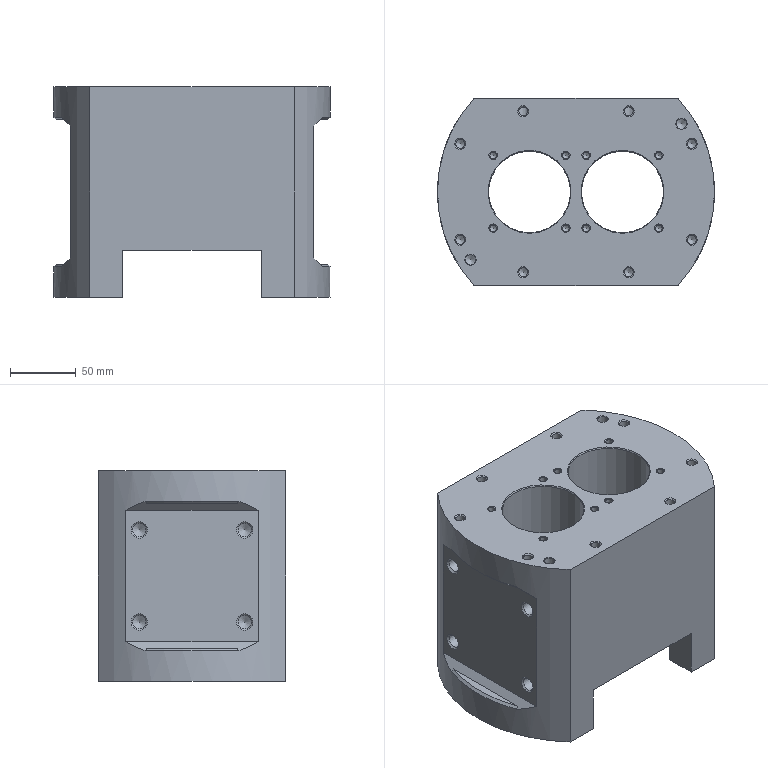NC program | NX | posted with a generic post | part box 210 x 142 x 160 mm
Whole program:
N10 G17 G21 G94 G90
(FLOOR_WALL , TOOL : D50)
N12 T02 M6
N14 G54
N16 G17 G0 G90 X-46.563 Y89.997 B0. C0. S1200 M3
N18 G43 Z30. H2
N20 Z2.65
N22 G94 G1 Z-0.35 F1000.
N24 X-43.563
N26 X43.563 F2000.
N28 Y49.998
N30 X-43.563
N32 Y9.999
N34 X43.563
N36 Y-30.001
N38 X-43.563
N40 Y-70.
N42 X43.563
N44 X46.563
N46 Z2.65
N48 G0 Z30.
N50 X-50.098 Y89.997
N52 Z2.301
N54 G1 Z-0.699 F1000.
N56 X-47.098
N58 X47.098 F2000.
N60 Y49.998
N62 X-47.098
N64 Y9.999
N66 X47.098
N68 Y-30.001
N70 X-47.098
N72 Y-70.
N74 X47.098
N76 X50.098
N78 Z2.301
N80 G0 Z30.
N82 X-52.803 Y89.997
N84 Z1.951
N86 G1 Z-1.049 F1000.
N88 X-49.803
N90 X49.803 F2000.
N92 Y49.998
N94 X-49.803
N96 Y9.999
N98 X49.803
N100 Y-30.001
N102 X-49.803
N104 Y-70.
N106 X49.803
N108 X52.803
N110 Z1.951
N112 G0 Z30.
N114 X-55.078 Y89.997
N116 Z1.602
N118 G1 Z-1.398 F1000.
N120 X-52.078
N122 X52.078 F2000.
N124 Y49.998
N126 X-52.078
N128 Y9.999
N130 X52.078
N132 Y-30.001
N134 X-52.078
N136 Y-70.
N138 X52.078
N140 X55.078
N142 Z1.602
N144 G0 Z30.
N146 X-57.078 Y89.997
N148 Z1.252
N150 G1 Z-1.748 F1000.
N152 X-54.078
N154 X54.078 F2000.
N156 Y49.998
N158 X-54.078
N160 Y9.999
N162 X54.078
N164 Y-30.001
N166 X-54.078
N168 Y-70.
N170 X54.078
N172 X57.078
N174 Z1.252
N176 G0 Z30.
N178 X-58.881 Y89.997
N180 Z0.903
N182 G1 Z-2.097 F1000.
N184 X-55.881
N186 X55.881 F2000.
N188 Y49.998
N190 X-55.881
N192 Y9.999
N194 X55.881
N196 Y-30.001
N198 X-55.881
N200 Y-70.
N202 X55.881
N204 X58.881
N206 Z0.903
N208 G0 Z30.
N210 X-60.535 Y89.997
N212 Z0.553
N214 G1 Z-2.447 F1000.
N216 X-57.535
N218 X57.535 F2000.
N220 Y49.998
N222 X-57.535
N224 Y9.999
N226 X57.535
N228 Y-30.001
N230 X-57.535
N232 Y-70.
N234 X57.535
N236 X60.535
N238 Z0.553
N240 G0 Z30.
N242 X-62.07 Y89.997
N244 Z0.204
N246 G1 Z-2.796 F1000.
N248 X-59.07
N250 X59.07 F2000.
N252 Y49.998
N254 X-59.07
N256 Y9.999
N258 X59.07
N260 Y-30.001
N262 X-59.07
N264 Y-70.
N266 X59.07
N268 X62.07
N270 Z0.204
N272 G0 Z30.
N274 X-63.509 Y89.997
N276 Z-0.146
N278 G1 Z-3.146 F1000.
N280 X-60.509
N282 X60.509 F2000.
N284 Y49.998
N286 X-60.509
N288 Y9.999
N290 X60.509
N292 Y-30.001
N294 X-60.509
N296 Y-70.
N298 X60.509
N300 X63.509
N302 Z-0.146
N304 G0 Z30.
N306 X-64.866 Y89.997
N308 Z-0.495
N310 G1 Z-3.495 F1000.
N312 X-61.866
N314 X61.866 F2000.
N316 Y49.998
N318 X-61.866
N320 Y9.999
N322 X61.866
N324 Y-30.001
N326 X-61.866
N328 Y-70.
N330 X61.866
N332 X64.866
N334 Z-0.495
N336 G0 Z30.
N338 X-66.153 Y89.997
N340 Z-0.845
N342 G1 Z-3.845 F1000.
N344 X-63.153
N346 X63.153 F2000.
N348 Y49.998
N350 X-63.153
N352 Y9.999
N354 X63.153
N356 Y-30.001
N358 X-63.153
N360 Y-70.
N362 X63.153
N364 X66.153
N366 Z-0.845
N368 G0 Z30.
N370 X-67.38 Y89.997
N372 Z-1.194
N374 G1 Z-4.194 F1000.
N376 X-64.38
N378 X64.38 F2000.
N380 Y49.998
N382 X-64.38
N384 Y9.999
N386 X64.38
N388 Y-30.001
N390 X-64.38
N392 Y-70.
N394 X64.38
N396 X67.38
N398 Z-1.194
N400 G0 Z30.
N402 X-68.553 Y89.997
N404 Z-1.544
N406 G1 Z-4.544 F1000.
N408 X-65.553
N410 X65.553 F2000.
N412 Y49.998
N414 X-65.553
N416 Y9.999
N418 X65.553
N420 Y-30.001
N422 X-65.553
N424 Y-70.
N426 X65.553
N428 X68.553
N430 Z-1.544
N432 G0 Z30.
N434 X-69.68 Y89.997
N436 Z-1.893
N438 G1 Z-4.893 F1000.
N440 X-66.68
N442 X66.68 F2000.
N444 Y49.998
N446 X-66.68
N448 Y9.999
N450 X66.68
N452 Y-30.001
N454 X-66.68
N456 Y-70.
N458 X66.68
N460 X69.68
N462 Z-1.893
N464 G0 Z30.
N466 X-70.763 Y89.997
N468 Z-2.243
N470 G1 Z-5.243 F1000.
N472 X-67.763
N474 X67.763 F2000.
N476 Y49.998
N478 X-67.763
N480 Y9.999
N482 X67.763
N484 Y-30.001
N486 X-67.763
N488 Y-70.
N490 X67.763
N492 X70.763
N494 Z-2.243
N496 G0 Z30.
N498 X-71.809 Y89.997
N500 Z-2.592
N502 G1 Z-5.592 F1000.
N504 X-68.809
N506 X68.809 F2000.
N508 Y49.998
N510 X-68.809
N512 Y9.999
N514 X68.809
N516 Y-30.001
N518 X-68.809
N520 Y-70.
N522 X68.809
N524 X71.809
N526 Z-2.592
N528 G0 Z30.
N530 X-72.82 Y89.997
N532 Z-2.941
N534 G1 Z-5.941 F1000.
N536 X-69.82
N538 X69.82 F2000.
N540 Y49.998
N542 X-69.82
N544 Y9.999
N546 X69.82
N548 Y-30.001
N550 X-69.82
N552 Y-70.
N554 X69.82
N556 X72.82
N558 Z-2.941
N560 G0 Z30.
N562 X-73.798 Y89.997
N564 Z-3.291
N566 G1 Z-6.291 F1000.
N568 X-70.798
N570 X70.798 F2000.
N572 Y49.998
N574 X-70.798
N576 Y9.999
N578 X70.798
N580 Y-30.001
N582 X-70.798
N584 Y-70.
N586 X70.798
N588 X73.798
N590 Z-3.291
N592 G0 Z30.
N594 X-74.748 Y89.997
N596 Z-3.64
N598 G1 Z-6.64 F1000.
N600 X-71.748
N602 X71.748 F2000.
N604 Y49.998
N606 X-71.748
N608 Y9.999
N610 X71.748
N612 Y-30.001
N614 X-71.748
N616 Y-70.
N618 X71.748
N620 X74.748
N622 Z-3.64
N624 G0 Z30.
N626 X-75.67 Y89.997
N628 Z-3.99
N630 G1 Z-6.99 F1000.
N632 X-72.67
N634 X72.67 F2000.
N636 Y49.998
N638 X-72.67
N640 Y9.999
N642 X72.67
N644 Y-30.001
N646 X-72.67
N648 Y-70.
N650 X72.67
N652 X75.67
N654 Z-3.99
N656 G0 Z30.
N658 X-76.567 Y89.997
N660 Z-4.339
N662 G1 Z-7.339 F1000.
N664 X-73.567
N666 X73.567 F2000.
N668 Y49.998
N670 X-73.567
N672 Y9.999
N674 X73.567
N676 Y-30.001
N678 X-73.567
N680 Y-70.
N682 X73.567
N684 X76.567
N686 Z-4.339
N688 G0 Z30.
N690 X-77.44 Y89.997
N692 Z-4.689
N694 G1 Z-7.689 F1000.
N696 X-74.44
N698 X74.44 F2000.
N700 Y49.998
N702 X-74.44
N704 Y9.999
N706 X74.44
N708 Y-30.001
N710 X-74.44
N712 Y-70.
N714 X74.44
N716 X77.44
N718 Z-4.689
N720 G0 Z30.
N722 X-78.292 Y89.997
N724 Z-5.038
N726 G1 Z-8.038 F1000.
N728 X-75.292
N730 X75.292 F2000.
N732 Y49.998
N734 X-75.292
N736 Y9.999
N738 X75.292
N740 Y-30.001
N742 X-75.292
N744 Y-70.
N746 X75.292
N748 X78.292
N750 Z-5.038
N752 G0 Z30.
N754 X-79.123 Y89.997
N756 Z-5.388
N758 G1 Z-8.388 F1000.
N760 X-76.123
N762 X76.123 F2000.
N764 Y49.998
N766 X-76.123
N768 Y9.999
N770 X76.123
N772 Y-30.001
N774 X-76.123
N776 Y-70.
N778 X76.123
N780 X79.123
N782 Z-5.388
N784 G0 Z30.
N786 X-79.934 Y89.997
N788 Z-5.737
N790 G1 Z-8.737 F1000.
N792 X-76.934
N794 X76.934 F2000.
N796 Y49.998
N798 X-76.934
N800 Y9.999
N802 X76.934
N804 Y-30.001
N806 X-76.934
N808 Y-70.
N810 X76.934
N812 X79.934
N814 Z-5.737
N816 G0 Z30.
N818 X-80.728 Y89.997
N820 Z-6.087
N822 G1 Z-9.087 F1000.
N824 X-77.728
N826 X77.728 F2000.
N828 Y49.998
N830 X-77.728
N832 Y9.999
N834 X77.728
N836 Y-30.001
N838 X-77.728
N840 Y-70.
N842 X77.728
N844 X80.728
N846 Z-6.087
N848 G0 Z30.
N850 X-81.504 Y89.997
N852 Z-6.436
N854 G1 Z-9.436 F1000.
N856 X-78.504
N858 X78.504 F2000.
N860 Y49.998
N862 X-78.504
N864 Y9.999
N866 X78.504
N868 Y-30.001
N870 X-78.504
N872 Y-70.
N874 X78.504
N876 X81.504
N878 Z-6.436
N880 G0 Z30.
N882 X-82.263 Y89.997
N884 Z-6.786
N886 G1 Z-9.786 F1000.
N888 X-79.263
N890 X79.263 F2000.
N892 Y49.998
N894 X-79.263
N896 Y9.999
N898 X79.263
N900 Y-30.001
N902 X-79.263
N904 Y-70.
N906 X79.263
N908 X82.263
N910 Z-6.786
N912 G0 Z30.
N914 X-83.008 Y89.997
N916 Z-7.135
N918 G1 Z-10.135 F1000.
N920 X-80.008
N922 X80.008 F2000.
N924 Y49.998
N926 X-80.008
N928 Y9.999
N930 X80.008
N932 Y-30.001
N934 X-80.008
N936 Y-70.
N938 X80.008
N940 X83.008
N942 Z-7.135
N944 G0 Z30.
N946 X-83.737 Y89.997
N948 Z-7.485
N950 G1 Z-10.485 F1000.
N952 X-80.737
N954 X80.737 F2000.
N956 Y49.998
N958 X-80.737
N960 Y9.999
N962 X80.737
N964 Y-30.001
N966 X-80.737
N968 Y-70.
N970 X80.737
N972 X83.737
N974 Z-7.485
N976 G0 Z30.
N978 X-84.452 Y89.997
N980 Z-7.834
N982 G1 Z-10.834 F1000.
N984 X-81.452
N986 X81.452 F2000.
N988 Y49.998
N990 X-81.452
N992 Y9.999
N994 X81.452
N996 Y-30.001
N998 X-81.452
N1000 Y-70.
N1002 X81.452
N1004 X84.452
N1006 Z-7.834
N1008 G0 Z30.
N1010 X-85.154 Y89.997
N1012 Z-8.184
N1014 G1 Z-11.184 F1000.
N1016 X-82.154
N1018 X82.154 F2000.
N1020 Y49.998
N1022 X-82.154
N1024 Y9.999
N1026 X82.154
N1028 Y-30.001
N1030 X-82.154
N1032 Y-70.
N1034 X82.154
N1036 X85.154
N1038 Z-8.184
N1040 G0 Z30.
N1042 X-85.843 Y89.997
N1044 Z-8.533
N1046 G1 Z-11.533 F1000.
N1048 X-82.843
N1050 X82.843 F2000.
N1052 Y49.998
N1054 X-82.843
N1056 Y9.999
N1058 X82.843
N1060 Y-30.001
N1062 X-82.843
N1064 Y-70.
N1066 X82.843
N1068 X85.843
N1070 Z-8.533
N1072 G0 Z30.
N1074 X-86.52 Y89.997
N1076 Z-8.883
N1078 G1 Z-11.883 F1000.
N1080 X-83.52
N1082 X83.52 F2000.
N1084 Y49.998
N1086 X-83.52
N1088 Y9.999
N1090 X83.52
N1092 Y-30.001
N1094 X-83.52
N1096 Y-70.
N1098 X83.52
N1100 X86.52
N1102 Z-8.883
N1104 G0 Z30.
N1106 X-87.185 Y89.997
N1108 Z-9.232
N1110 G1 Z-12.232 F1000.
N1112 X-84.185
N1114 X84.185 F2000.
N1116 Y49.998
N1118 X-84.185
N1120 Y9.999
N1122 X84.185
N1124 Y-30.001
N1126 X-84.185
N1128 Y-70.
N1130 X84.185
N1132 X87.185
N1134 Z-9.232
N1136 G0 Z30.
N1138 X-87.838 Y89.997
N1140 Z-9.582
N1142 G1 Z-12.582 F1000.
N1144 X-84.838
N1146 X84.838 F2000.
N1148 Y49.998
N1150 X-84.838
N1152 Y9.999
N1154 X84.838
N1156 Y-30.001
N1158 X-84.838
N1160 Y-70.
N1162 X84.838
N1164 X87.838
N1166 Z-9.582
N1168 G0 Z30.
N1170 X-88.481 Y89.997
N1172 Z-9.931
N1174 G1 Z-12.931 F1000.
N1176 X-85.481
N1178 X85.481 F2000.
N1180 Y49.998
N1182 X-85.481
N1184 Y9.999
N1186 X85.481
N1188 Y-30.001
N1190 X-85.481
N1192 Y-70.
N1194 X85.481
N1196 X88.481
N1198 Z-9.931
N1200 G0 Z30.
N1202 X-89.113 Y89.997
N1204 Z-10.281
N1206 G1 Z-13.281 F1000.
N1208 X-86.113
N1210 X86.113 F2000.
N1212 Y49.998
N1214 X-86.113
N1216 Y9.999
N1218 X86.113
N1220 Y-30.001
N1222 X-86.113
N1224 Y-70.
N1226 X86.113
N1228 X89.113
N1230 Z-10.281
N1232 G0 Z30.
N1234 X-89.735 Y89.997
N1236 Z-10.63
N1238 G1 Z-13.63 F1000.
N1240 X-86.735
N1242 X86.735 F2000.
N1244 Y49.998
N1246 X-86.735
N1248 Y9.999
N1250 X86.735
N1252 Y-30.001
N1254 X-86.735
N1256 Y-70.
N1258 X86.735
N1260 X89.735
N1262 Z-10.63
N1264 G0 Z30.
N1266 X-90.348 Y89.997
N1268 Z-10.98
N1270 G1 Z-13.98 F1000.
N1272 X-87.348
N1274 X87.348 F2000.
N1276 Y49.998
N1278 X-87.348
N1280 Y9.999
N1282 X87.348
N1284 Y-30.001
N1286 X-87.348
N1288 Y-70.
N1290 X87.348
N1292 X90.348
N1294 Z-10.98
N1296 G0 Z30.
N1298 X-90.951 Y89.997
N1300 Z-11.329
N1302 G1 Z-14.329 F1000.
N1304 X-87.951
N1306 X87.951 F2000.
N1308 Y49.998
N1310 X-87.951
N1312 Y9.999
N1314 X87.951
N1316 Y-30.001
N1318 X-87.951
N1320 Y-70.
N1322 X87.951
N1324 X90.951
N1326 Z-11.329
N1328 G0 Z30.
N1330 X-91.545 Y89.997
N1332 Z-11.679
N1334 G1 Z-14.679 F1000.
N1336 X-88.545
N1338 X88.545 F2000.
N1340 Y49.998
N1342 X-88.545
N1344 Y9.999
N1346 X88.545
N1348 Y-30.001
N1350 X-88.545
N1352 Y-70.
N1354 X88.545
N1356 X91.545
N1358 Z-11.679
N1360 G0 Z30.
N1362 X-92.13 Y89.997
N1364 Z-12.028
N1366 G1 Z-15.028 F1000.
N1368 X-89.13
N1370 X89.13 F2000.
N1372 Y49.998
N1374 X-89.13
N1376 Y9.999
N1378 X89.13
N1380 Y-30.001
N1382 X-89.13
N1384 Y-70.
N1386 X89.13
N1388 X92.13
N1390 Z-12.028
N1392 G0 Z30.
N1394 X-92.707 Y89.997
N1396 Z-12.377
N1398 G1 Z-15.377 F1000.
N1400 X-89.707
N1402 X89.707 F2000.
N1404 Y49.998
N1406 X-89.707
N1408 Y9.999
N1410 X89.707
N1412 Y-30.001
N1414 X-89.707
N1416 Y-70.
N1418 X89.707
N1420 X92.707
N1422 Z-12.377
N1424 G0 Z30.
N1426 X-93.275 Y89.997
N1428 Z-12.727
N1430 G1 Z-15.727 F1000.
N1432 X-90.275
N1434 X90.275 F2000.
N1436 Y49.998
N1438 X-90.275
N1440 Y9.999
N1442 X90.275
N1444 Y-30.001
N1446 X-90.275
N1448 Y-70.
N1450 X90.275
N1452 X93.275
N1454 Z-12.727
N1456 G0 Z30.
N1458 X-93.835 Y89.997
N1460 Z-13.076
N1462 G1 Z-16.076 F1000.
N1464 X-90.835
N1466 X90.835 F2000.
N1468 Y49.998
N1470 X-90.835
N1472 Y9.999
N1474 X90.835
N1476 Y-30.001
N1478 X-90.835
N1480 Y-70.
N1482 X90.835
N1484 X93.835
N1486 Z-13.076
N1488 G0 Z30.
N1490 X-94.388 Y89.997
N1492 Z-13.426
N1494 G1 Z-16.426 F1000.
N1496 X-91.388
N1498 X91.388 F2000.
N1500 Y49.998
N1502 X-91.388
N1504 Y9.999
N1506 X91.388
N1508 Y-30.001
N1510 X-91.388
N1512 Y-70.
N1514 X91.388
N1516 X94.388
N1518 Z-13.426
N1520 G0 Z30.
N1522 X-94.933 Y89.997
N1524 Z-13.775
N1526 G1 Z-16.775 F1000.
N1528 X-91.933
N1530 X91.933 F2000.
N1532 Y49.998
N1534 X-91.933
N1536 Y9.999
N1538 X91.933
N1540 Y-30.001
N1542 X-91.933
N1544 Y-70.
N1546 X91.933
N1548 X94.933
N1550 Z-13.775
N1552 G0 Z30.
N1554 X-95.471 Y89.997
N1556 Z-14.125
N1558 G1 Z-17.125 F1000.
N1560 X-92.471
N1562 X92.471 F2000.
N1564 Y49.998
N1566 X-92.471
N1568 Y9.999
N1570 X92.471
N1572 Y-30.001
N1574 X-92.471
N1576 Y-70.
N1578 X92.471
N1580 X95.471
N1582 Z-14.125
N1584 G0 Z30.
N1586 X-96.002 Y89.997
N1588 Z-14.474
N1590 G1 Z-17.474 F1000.
N1592 X-93.002
N1594 X93.002 F2000.
N1596 Y49.998
N1598 X-93.002
N1600 Y9.999
N1602 X93.002
N1604 Y-30.001
N1606 X-93.002
N1608 Y-70.
N1610 X93.002
N1612 X96.002
N1614 Z-14.474
N1616 G0 Z30.
N1618 X-96.526 Y89.997
N1620 Z-14.824
N1622 G1 Z-17.824 F1000.
N1624 X-93.526
N1626 X93.526 F2000.
N1628 Y49.998
N1630 X-93.526
N1632 Y9.999
N1634 X93.526
N1636 Y-30.001
N1638 X-93.526
N1640 Y-70.
N1642 X93.526
N1644 X96.526
N1646 Z-14.824
N1648 G0 Z30.
N1650 X-97.043 Y89.997
N1652 Z-15.173
N1654 G1 Z-18.173 F1000.
N1656 X-94.043
N1658 X94.043 F2000.
N1660 Y49.998
N1662 X-94.043
N1664 Y9.999
N1666 X94.043
N1668 Y-30.001
N1670 X-94.043
N1672 Y-70.
N1674 X94.043
N1676 X97.043
N1678 Z-15.173
N1680 G0 Z30.
N1682 X-97.554 Y89.997
N1684 Z-15.523
N1686 G1 Z-18.523 F1000.
N1688 X-94.554
N1690 X94.554 F2000.
N1692 Y49.998
N1694 X-94.554
N1696 Y9.999
N1698 X94.554
N1700 Y-30.001
N1702 X-94.554
N1704 Y-70.
N1706 X94.554
N1708 X97.554
N1710 Z-15.523
N1712 G0 Z30.
N1714 X-98.058 Y89.997
N1716 Z-15.872
N1718 G1 Z-18.872 F1000.
N1720 X-95.058
N1722 X95.058 F2000.
N1724 Y49.998
N1726 X-95.058
N1728 Y9.999
N1730 X95.058
N1732 Y-30.001
N1734 X-95.058
N1736 Y-70.
N1738 X95.058
N1740 X98.058
N1742 Z-15.872
N1744 G0 Z30.
N1746 X-98.557 Y89.997
N1748 Z-16.222
N1750 G1 Z-19.222 F1000.
N1752 X-95.557
N1754 X95.557 F2000.
N1756 Y49.998
N1758 X-95.557
N1760 Y9.999
N1762 X95.557
N1764 Y-30.001
N1766 X-95.557
N1768 Y-70.
N1770 X95.557
N1772 X98.557
N1774 Z-16.222
N1776 G0 Z30.
N1778 X-99.049 Y89.997
N1780 Z-16.571
N1782 G1 Z-19.571 F1000.
N1784 X-96.049
N1786 X96.049 F2000.
N1788 Y49.998
N1790 X-96.049
N1792 Y9.999
N1794 X96.049
N1796 Y-30.001
N1798 X-96.049
N1800 Y-70.
N1802 X96.049
N1804 X99.049
N1806 Z-16.571
N1808 G0 Z30.
N1810 X-99.535 Y89.997
N1812 Z-16.921
N1814 G1 Z-19.921 F1000.
N1816 X-96.535
N1818 X96.535 F2000.
N1820 Y49.998
N1822 X-96.535
N1824 Y9.999
N1826 X96.535
N1828 Y-30.001
N1830 X-96.535
N1832 Y-70.
N1834 X96.535
N1836 X99.535
N1838 Z-16.921
N1840 G0 Z30.
N1842 X-100.015 Y89.997
N1844 Z-17.27
N1846 G1 Z-20.27 F1000.
N1848 X-97.015
N1850 X97.015 F2000.
N1852 Y49.998
N1854 X-97.015
N1856 Y9.999
N1858 X97.015
N1860 Y-30.001
N1862 X-97.015
N1864 Y-70.
N1866 X97.015
N1868 X100.015
N1870 Z-17.27
N1872 G0 Z30.
N1874 X-100.49 Y89.997
N1876 Z-17.62
N1878 G1 Z-20.62 F1000.
N1880 X-97.49
N1882 X97.49 F2000.
N1884 Y49.998
N1886 X-97.49
N1888 Y9.999
N1890 X97.49
N1892 Y-30.001
N1894 X-97.49
N1896 Y-70.
N1898 X97.49
N1900 X100.49
N1902 Z-17.62
N1904 G0 Z30.
N1906 X-100.959 Y89.997
N1908 Z-17.969
N1910 G1 Z-20.969 F1000.
N1912 X-97.959
N1914 X97.959 F2000.
N1916 Y49.998
N1918 X-97.959
N1920 Y9.999
N1922 X97.959
N1924 Y-30.001
N1926 X-97.959
N1928 Y-70.
N1930 X97.959
N1932 X100.959
N1934 Z-17.969
N1936 G0 Z30.
N1938 X-101.423 Y89.997
N1940 Z-18.319
N1942 G1 Z-21.319 F1000.
N1944 X-98.423
N1946 X98.423 F2000.
N1948 Y49.998
N1950 X-98.423
N1952 Y9.999
N1954 X98.423
N1956 Y-30.001
N1958 X-98.423
N1960 Y-70.
N1962 X98.423
N1964 X101.423
N1966 Z-18.319
N1968 G0 Z30.
N1970 X-101.881 Y89.997
N1972 Z-18.668
N1974 G1 Z-21.668 F1000.
N1976 X-98.881
N1978 X98.881 F2000.
N1980 Y49.998
N1982 X-98.881
N1984 Y9.999
N1986 X98.881
N1988 Y-30.001
N1990 X-98.881
N1992 Y-70.
N1994 X98.881
N1996 X101.881
N1998 Z-18.668
N2000 G0 Z30.
N2002 X-102.334 Y89.997
N2004 Z-19.018
N2006 G1 Z-22.018 F1000.
N2008 X-99.334
N2010 X99.334 F2000.
N2012 Y49.998
N2014 X-99.334
N2016 Y9.999
N2018 X99.334
N2020 Y-30.001
N2022 X-99.334
N2024 Y-70.
N2026 X99.334
N2028 X102.334
N2030 Z-19.018
N2032 G0 Z30.
N2034 X-102.783 Y89.997
N2036 Z-19.367
N2038 G1 Z-22.367 F1000.
N2040 X-99.783
N2042 X99.783 F2000.
N2044 Y49.998
N2046 X-99.783
N2048 Y9.999
N2050 X99.783
N2052 Y-30.001
N2054 X-99.783
N2056 Y-70.
N2058 X99.783
N2060 X102.783
N2062 Z-19.367
N2064 G0 Z30.
N2066 X-103.226 Y89.997
N2068 Z-19.717
N2070 G1 Z-22.717 F1000.
N2072 X-100.226
N2074 X100.226 F2000.
N2076 Y49.998
N2078 X-100.226
N2080 Y9.999
N2082 X100.226
N2084 Y-30.001
N2086 X-100.226
N2088 Y-70.
N2090 X100.226
N2092 X103.226
N2094 Z-19.717
N2096 G0 Z30.
N2098 X-103.665 Y89.997
N2100 Z-20.066
N2102 G1 Z-23.066 F1000.
N2104 X-100.665
N2106 X100.665 F2000.
N2108 Y49.998
N2110 X-100.665
N2112 Y9.999
N2114 X100.665
N2116 Y-30.001
N2118 X-100.665
N2120 Y-70.
N2122 X100.665
N2124 X103.665
N2126 Z-20.066
N2128 G0 Z30.
N2130 X-104.098 Y89.997
N2132 Z-20.416
N2134 G1 Z-23.416 F1000.
N2136 X-101.098
N2138 X101.098 F2000.
N2140 Y49.998
N2142 X-101.098
N2144 Y9.999
N2146 X101.098
N2148 Y-30.001
N2150 X-101.098
N2152 Y-70.
N2154 X101.098
N2156 X104.098
N2158 Z-20.416
N2160 G0 Z30.
N2162 X-104.527 Y89.997
N2164 Z-20.765
N2166 G1 Z-23.765 F1000.
N2168 X-101.527
N2170 X101.527 F2000.
N2172 Y49.998
N2174 X-101.527
N2176 Y9.999
N2178 X101.527
N2180 Y-30.001
N2182 X-101.527
N2184 Y-70.
N2186 X101.527
N2188 X104.527
N2190 Z-20.765
N2192 G0 Z30.
N2194 X-104.952 Y89.997
N2196 Z-21.115
N2198 G1 Z-24.115 F1000.
N2200 X-101.952
N2202 X101.952 F2000.
N2204 Y49.998
N2206 X-101.952
N2208 Y9.999
N2210 X101.952
N2212 Y-30.001
N2214 X-101.952
N2216 Y-70.
N2218 X101.952
N2220 X104.952
N2222 Z-21.115
N2224 G0 Z30.
N2226 X-105.372 Y89.997
N2228 Z-21.464
N2230 G1 Z-24.464 F1000.
N2232 X-102.372
N2234 X102.372 F2000.
N2236 Y49.998
N2238 X-102.372
N2240 Y9.999
N2242 X102.372
N2244 Y-30.001
N2246 X-102.372
N2248 Y-70.
N2250 X102.372
N2252 X105.372
N2254 Z-21.464
N2256 G0 Z30.
N2258 X-105.787 Y89.997
N2260 Z-21.813
N2262 G1 Z-24.813 F1000.
N2264 X-102.787
N2266 X102.787 F2000.
N2268 Y49.998
N2270 X-102.787
N2272 Y9.999
N2274 X102.787
N2276 Y-30.001
N2278 X-102.787
N2280 Y-70.
N2282 X102.787
N2284 X105.787
N2286 Z-21.813
N2288 G0 Z30.
N2290 X-106.199 Y89.997
N2292 Z-22.163
N2294 G1 Z-25.163 F1000.
N2296 X-103.199
N2298 X103.199 F2000.
N2300 Y49.998
N2302 X-103.199
N2304 Y9.999
N2306 X103.199
N2308 Y-30.001
N2310 X-103.199
N2312 Y-70.
N2314 X103.199
N2316 X106.199
N2318 Z-22.163
N2320 G0 Z30.
N2322 X-106.606 Y89.997
N2324 Z-22.512
N2326 G1 Z-25.512 F1000.
N2328 X-103.606
N2330 X103.606 F2000.
N2332 Y49.998
N2334 X-103.606
N2336 Y9.999
N2338 X103.606
N2340 Y-30.001
N2342 X-103.606
N2344 Y-70.
N2346 X103.606
N2348 X106.606
N2350 Z-22.512
N2352 G0 Z30.
N2354 X-107.008 Y89.997
N2356 Z-22.862
N2358 G1 Z-25.862 F1000.
N2360 X-104.008
N2362 X104.008 F2000.
N2364 Y49.998
N2366 X-104.008
N2368 Y9.999
N2370 X104.008
N2372 Y-30.001
N2374 X-104.008
N2376 Y-70.
N2378 X104.008
N2380 X107.008
N2382 Z-22.862
N2384 G0 Z30.
N2386 X-107.407 Y89.997
N2388 Z-23.211
N2390 G1 Z-26.211 F1000.
N2392 X-104.407
N2394 X104.407 F2000.
N2396 Y49.998
N2398 X-104.407
N2400 Y9.999
N2402 X104.407
N2404 Y-30.001
N2406 X-104.407
N2408 Y-70.
N2410 X104.407
N2412 X107.407
N2414 Z-23.211
N2416 G0 Z30.
N2418 X-107.802 Y89.997
N2420 Z-23.561
N2422 G1 Z-26.561 F1000.
N2424 X-104.802
N2426 X104.802 F2000.
N2428 Y49.998
N2430 X-104.802
N2432 Y9.999
N2434 X104.802
N2436 Y-30.001
N2438 X-104.802
N2440 Y-70.
N2442 X104.802
N2444 X107.802
N2446 Z-23.561
N2448 G0 Z30.
N2450 X-108.193 Y89.997
N2452 Z-23.91
N2454 G1 Z-26.91 F1000.
N2456 X-105.193
N2458 X105.193 F2000.
N2460 Y49.998
N2462 X-105.193
N2464 Y9.999
N2466 X105.193
N2468 Y-30.001
N2470 X-105.193
N2472 Y-70.
N2474 X105.193
N2476 X108.193
N2478 Z-23.91
N2480 G0 Z30.
N2482 X-108.58 Y89.997
N2484 Z-24.26
N2486 G1 Z-27.26 F1000.
N2488 X-105.58
N2490 X105.58 F2000.
N2492 Y49.998
N2494 X-105.58
N2496 Y9.999
N2498 X105.58
N2500 Y-30.001
N2502 X-105.58
N2504 Y-70.
N2506 X105.58
N2508 X108.58
N2510 Z-24.26
N2512 G0 Z30.
N2514 X-108.963 Y89.997
N2516 Z-24.609
N2518 G1 Z-27.609 F1000.
N2520 X-105.963
N2522 X105.963 F2000.
N2524 Y49.998
N2526 X-105.963
N2528 Y9.999
N2530 X105.963
N2532 Y-30.001
N2534 X-105.963
N2536 Y-70.
N2538 X105.963
N2540 X108.963
N2542 Z-24.609
N2544 G0 Z30.
N2546 X-109.342 Y89.997
N2548 Z-24.959
N2550 G1 Z-27.959 F1000.
N2552 X-106.342
N2554 X106.342 F2000.
N2556 Y49.998
N2558 X-106.342
N2560 Y9.999
N2562 X106.342
N2564 Y-30.001
N2566 X-106.342
N2568 Y-70.
N2570 X106.342
N2572 X109.342
N2574 Z-24.959
N2576 G0 Z30.
N2578 X-109.717 Y89.997
N2580 Z-25.308
N2582 G1 Z-28.308 F1000.
N2584 X-106.717
N2586 X106.717 F2000.
N2588 Y49.998
N2590 X-106.717
N2592 Y9.999
N2594 X106.717
N2596 Y-30.001
N2598 X-106.717
N2600 Y-70.
N2602 X106.717
N2604 X109.717
N2606 Z-25.308
N2608 G0 Z30.
N2610 X-110.089 Y89.997
N2612 Z-25.658
N2614 G1 Z-28.658 F1000.
N2616 X-107.089
N2618 X107.089 F2000.
N2620 Y49.998
N2622 X-107.089
N2624 Y9.999
N2626 X107.089
N2628 Y-30.001
N2630 X-107.089
N2632 Y-70.
N2634 X107.089
N2636 X110.089
N2638 Z-25.658
N2640 G0 Z30.
N2642 X-110.458 Y89.997
N2644 Z-26.007
N2646 G1 Z-29.007 F1000.
N2648 X-107.458
N2650 X107.458 F2000.
N2652 Y49.998
N2654 X-107.458
N2656 Y9.999
N2658 X107.458
N2660 Y-30.001
N2662 X-107.458
N2664 Y-70.
N2666 X107.458
N2668 X110.458
N2670 Z-26.007
N2672 G0 Z30.
N2674 X-110.822 Y89.997
N2676 Z-26.357
N2678 G1 Z-29.357 F1000.
N2680 X-107.822
N2682 X107.822 F2000.
N2684 Y49.998
N2686 X-107.822
N2688 Y9.999
N2690 X107.822
N2692 Y-30.001
N2694 X-107.822
N2696 Y-70.
N2698 X107.822
N2700 X110.822
N2702 Z-26.357
N2704 G0 Z30.
N2706 X-111.184 Y89.997
N2708 Z-26.706
N2710 G1 Z-29.706 F1000.
N2712 X-108.184
N2714 X108.184 F2000.
N2716 Y49.998
N2718 X-108.184
N2720 Y9.999
N2722 X108.184
N2724 Y-30.001
N2726 X-108.184
N2728 Y-70.
N2730 X108.184
N2732 X111.184
N2734 Z-26.706
N2736 G0 Z30.
N2738 X-111.542 Y89.997
N2740 Z-27.056
N2742 G1 Z-30.056 F1000.
N2744 X-108.542
N2746 X108.542 F2000.
N2748 Y49.998
N2750 X-108.542
N2752 Y9.999
N2754 X108.542
N2756 Y-30.001
N2758 X-108.542
N2760 Y-70.
N2762 X108.542
N2764 X111.542
N2766 Z-27.056
N2768 G0 Z30.
N2770 X-111.896 Y89.997
N2772 Z-27.405
N2774 G1 Z-30.405 F1000.
N2776 X-108.896
N2778 X108.896 F2000.
N2780 Y49.998
N2782 X-108.896
N2784 Y9.999
N2786 X108.896
N2788 Y-30.001
N2790 X-108.896
N2792 Y-70.
N2794 X108.896
N2796 X111.896
N2798 Z-27.405
N2800 G0 Z30.
N2802 X-112.247 Y89.997
N2804 Z-27.755
N2806 G1 Z-30.755 F1000.
N2808 X-109.247
N2810 X109.247 F2000.
N2812 Y49.998
N2814 X-109.247
N2816 Y9.999
N2818 X109.247
N2820 Y-30.001
N2822 X-109.247
N2824 Y-70.
N2826 X109.247
N2828 X112.247
N2830 Z-27.755
N2832 G0 Z30.
N2834 X-112.595 Y89.997
N2836 Z-28.104
N2838 G1 Z-31.104 F1000.
N2840 X-109.595
N2842 X109.595 F2000.
N2844 Y49.998
N2846 X-109.595
N2848 Y9.999
N2850 X109.595
N2852 Y-30.001
N2854 X-109.595
N2856 Y-70.
N2858 X109.595
N2860 X112.595
N2862 Z-28.104
N2864 G0 Z30.
N2866 X-112.94 Y89.997
N2868 Z-28.454
N2870 G1 Z-31.454 F1000.
N2872 X-109.94
N2874 X109.94 F2000.
N2876 Y49.998
N2878 X-109.94
N2880 Y9.999
N2882 X109.94
N2884 Y-30.001
N2886 X-109.94
N2888 Y-70.
N2890 X109.94
N2892 X112.94
N2894 Z-28.454
N2896 G0 Z30.
N2898 X-113.281 Y89.997
N2900 Z-28.803
N2902 G1 Z-31.803 F1000.
N2904 X-110.281
N2906 X110.281 F2000.
N2908 Y49.998
N2910 X-110.281
N2912 Y9.999
N2914 X110.281
N2916 Y-30.001
N2918 X-110.281
N2920 Y-70.
N2922 X110.281
N2924 X113.281
N2926 Z-28.803
N2928 G0 Z30.
N2930 X-113.619 Y89.997
N2932 Z-29.153
N2934 G1 Z-32.153 F1000.
N2936 X-110.619
N2938 X110.619 F2000.
N2940 Y49.998
N2942 X-110.619
N2944 Y9.999
N2946 X110.619
N2948 Y-30.001
N2950 X-110.619
N2952 Y-70.
N2954 X110.619
N2956 X113.619
N2958 Z-29.153
N2960 G0 Z30.
N2962 X-113.954 Y89.997
N2964 Z-29.502
N2966 G1 Z-32.502 F1000.
N2968 X-110.954
N2970 X110.954 F2000.
N2972 Y49.998
N2974 X-110.954
N2976 Y9.999
N2978 X110.954
N2980 Y-30.001
N2982 X-110.954
N2984 Y-70.
N2986 X110.954
N2988 X113.954
N2990 Z-29.502
N2992 G0 Z30.
N2994 X-114.286 Y89.997
N2996 Z-29.852
N2998 G1 Z-32.852 F1000.
N3000 X-111.286
N3002 X111.286 F2000.
N3004 Y49.998
N3006 X-111.286
N3008 Y9.999
N3010 X111.286
N3012 Y-30.001
N3014 X-111.286
N3016 Y-70.
N3018 X111.286
N3020 X114.286
N3022 Z-29.852
N3024 G0 Z30.
N3026 X-114.615 Y89.997
N3028 Z-30.201
N3030 G1 Z-33.201 F1000.
N3032 X-111.615
N3034 X111.615 F2000.
N3036 Y49.998
N3038 X-111.615
N3040 Y9.999
N3042 X111.615
N3044 Y-30.001
N3046 X-111.615
N3048 Y-70.
N3050 X111.615
N3052 X114.615
N3054 Z-30.201
N3056 G0 Z30.
N3058 X-114.941 Y89.997
N3060 Z-30.551
N3062 G1 Z-33.551 F1000.
N3064 X-111.941
N3066 X111.941 F2000.
N3068 Y49.998
N3070 X-111.941
N3072 Y9.999
N3074 X111.941
N3076 Y-30.001
N3078 X-111.941
N3080 Y-70.
N3082 X111.941
N3084 X114.941
N3086 Z-30.551
N3088 G0 Z30.
N3090 X-115.264 Y89.997
N3092 Z-30.9
N3094 G1 Z-33.9 F1000.
N3096 X-112.264
N3098 X112.264 F2000.
N3100 Y49.998
N3102 X-112.264
N3104 Y9.999
N3106 X112.264
N3108 Y-30.001
N3110 X-112.264
N3112 Y-70.
N3114 X112.264
N3116 X115.264
N3118 Z-30.9
N3120 G0 Z30.
(FLOOR_WALL_COPY , TOOL : D50)
N3122 X-115.356 Y89.997 S2500
N3124 Z-31.
N3126 G1 Z-34. F1000.
N3128 X-112.356
N3130 X112.356
N3132 Y80.
N3134 Y49.998
N3136 X-112.356
N3138 Y9.999
N3140 X112.356
N3142 Y-30.001
N3144 X-112.356
N3146 Y-70.
N3148 X112.356
N3150 X115.356
N3152 Z-31.
N3154 G0 Z30.
N3156 M5
(DRILLING , TOOL : ZXZ)
N3158 T01 M6
N3160 G54
N3162 G17 G0 G90 X40. Y15. B0. C0. S5000 M3
N3164 G43 Z30. H1
N3166 G94 G81 G98 Z-35. F250. R-31.
N3168 Y-55.
N3170 X-40.
N3172 Y15.
N3174 G80
N3176 G0 X-40. Y15. Z30.
N3178 M5
(DRILLING_COPY , TOOL : 10.2ZT)
N3180 T11 M6
N3182 G54
N3184 G17 G0 G90 X40. Y15. B0. C0. S1200 M3
N3186 G43 Z30. H11
N3188 G94 G83 G98 Z-63.064 F250. Q2. R-31.
N3190 Y-55.
N3192 X-40. Y15.
N3194 Y-55.
N3196 G80
N3198 G0 X-40. Y-55. Z30.
N3200 M5
(PLANAR_MILL_COPY_COPY , TOOL : D6A45)
N3202 T07 M6
N3204 G54
N3206 G17 G0 G90 X42.947 Y13.021 B0. C0. S7500 M3
N3208 G43 Z30. H7
N3210 Z-32.5
N3212 G94 G1 Z-35.5 F1250.
N3214 X44.393 Y14.234
N3216 G3 X44.75 Y15. R1.
N3218 X40. Y19.75 R4.75
N3220 X44.75 Y15. R-4.75
N3222 X44.393 Y15.766 R1.
N3224 G1 X42.947 Y16.979
N3226 Z-32.5
N3228 G0 Z30.
N3230 X38.021 Y-57.947
N3232 Z-32.5
N3234 G1 Z-35.5
N3236 X39.234 Y-59.393
N3238 G3 X40. Y-59.75 R1.
N3240 X44.75 Y-55. R4.75
N3242 X40. Y-59.75 R-4.75
N3244 X40.766 Y-59.393 R1.
N3246 G1 X41.979 Y-57.947
N3248 Z-32.5
N3250 G0 Z30.
N3252 X-41.979
N3254 Z-32.5
N3256 G1 Z-35.5
N3258 X-40.766 Y-59.393
N3260 G3 X-40. Y-59.75 R1.
N3262 X-35.25 Y-55. R4.75
N3264 X-40. Y-59.75 R-4.75
N3266 X-39.234 Y-59.393 R1.
N3268 G1 X-38.021 Y-57.947
N3270 Z-32.5
N3272 G0 Z30.
N3274 X-42.947 Y16.979
N3276 Z-32.5
N3278 G1 Z-35.5
N3280 X-44.393 Y15.766
N3282 G3 X-44.75 Y15. R1.
N3284 X-40. Y10.25 R4.75
N3286 X-44.75 Y15. R-4.75
N3288 X-44.393 Y14.234 R1.
N3290 G1 X-42.947 Y13.021
N3292 Z-32.5
N3294 G0 Z30.
N3296 M5
N3298 M2